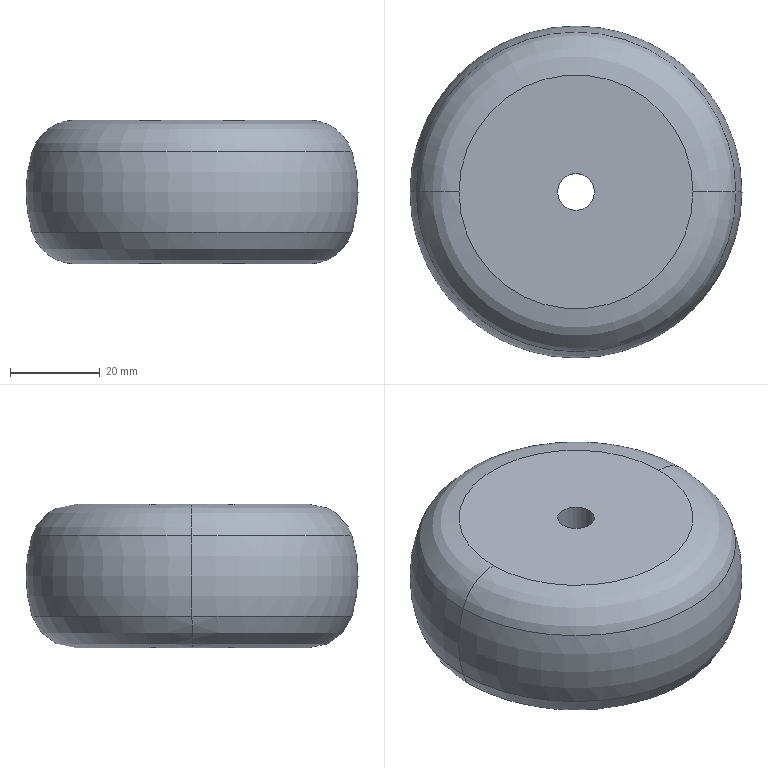Part | SolidWorks | features Fillet 1, Revolution 1 | 1 solid | 10 faces | box 74 x 74 x 32 mm | volume 122167 mm3 | torus 6 | cylinder 2 | plane 2 | commonest cylinder face diameters 8.2 x2
STEP:
#1=CARTESIAN_POINT('',(-35.618,0.,9.));
#2=VERTEX_POINT('',#1);
#3=CARTESIAN_POINT('',(35.618,0.,9.));
#4=VERTEX_POINT('',#3);
#5=CARTESIAN_POINT('',(0.,0.,9.));
#6=DIRECTION('',(0.,0.,-1.));
#7=DIRECTION('',(-1.,0.,0.));
#8=AXIS2_PLACEMENT_3D('',#5,#6,#7);
#9=CIRCLE('',#8,35.618);
#10=EDGE_CURVE('',#2,#4,#9,.T.);
#11=ORIENTED_EDGE('',*,*,#10,.F.);
#12=CARTESIAN_POINT('',(-26.079,0.,16.));
#13=VERTEX_POINT('',#12);
#14=CARTESIAN_POINT('',(-26.079,0.,6.));
#15=DIRECTION('',(0.,1.,0.));
#16=DIRECTION('',(-1.,0.,0.));
#17=AXIS2_PLACEMENT_3D('',#14,#15,#16);
#18=CIRCLE('',#17,10.);
#19=EDGE_CURVE('',#2,#13,#18,.T.);
#20=ORIENTED_EDGE('',*,*,#19,.T.);
#21=CARTESIAN_POINT('',(26.079,0.,16.));
#22=VERTEX_POINT('',#21);
#23=CARTESIAN_POINT('',(0.,0.,16.));
#24=DIRECTION('',(0.,0.,1.));
#25=DIRECTION('',(1.,0.,0.));
#26=AXIS2_PLACEMENT_3D('',#23,#24,#25);
#27=CIRCLE('',#26,26.079);
#28=EDGE_CURVE('',#22,#13,#27,.T.);
#29=ORIENTED_EDGE('',*,*,#28,.F.);
#30=CARTESIAN_POINT('',(26.079,0.,6.));
#31=DIRECTION('',(0.,-1.,0.));
#32=DIRECTION('',(0.,0.,-1.));
#33=AXIS2_PLACEMENT_3D('',#30,#31,#32);
#34=CIRCLE('',#33,10.);
#35=EDGE_CURVE('',#4,#22,#34,.T.);
#36=ORIENTED_EDGE('',*,*,#35,.F.);
#37=EDGE_LOOP('',(#11,#20,#29,#36));
#38=FACE_OUTER_BOUND('',#37,.T.);
#39=CARTESIAN_POINT('',(0.,0.,6.));
#40=DIRECTION('',(0.,0.,1.));
#41=DIRECTION('',(1.,0.,0.));
#42=AXIS2_PLACEMENT_3D('',#39,#40,#41);
#43=TOROIDAL_SURFACE('',#42,26.079,10.);
#44=ADVANCED_FACE('',(#38),#43,.T.);
#45=CARTESIAN_POINT('',(35.618,0.,-9.));
#46=VERTEX_POINT('',#45);
#47=CARTESIAN_POINT('',(-35.618,0.,-9.));
#48=VERTEX_POINT('',#47);
#49=CARTESIAN_POINT('',(0.,0.,-9.));
#50=DIRECTION('',(0.,0.,1.));
#51=DIRECTION('',(1.,0.,0.));
#52=AXIS2_PLACEMENT_3D('',#49,#50,#51);
#53=CIRCLE('',#52,35.618);
#54=EDGE_CURVE('',#46,#48,#53,.T.);
#55=ORIENTED_EDGE('',*,*,#54,.F.);
#56=CARTESIAN_POINT('',(26.079,0.,-16.));
#57=VERTEX_POINT('',#56);
#58=CARTESIAN_POINT('',(26.079,0.,-6.));
#59=DIRECTION('',(0.,1.,0.));
#60=DIRECTION('',(-1.,0.,0.));
#61=AXIS2_PLACEMENT_3D('',#58,#59,#60);
#62=CIRCLE('',#61,10.);
#63=EDGE_CURVE('',#46,#57,#62,.T.);
#64=ORIENTED_EDGE('',*,*,#63,.T.);
#65=CARTESIAN_POINT('',(-26.079,0.,-16.));
#66=VERTEX_POINT('',#65);
#67=CARTESIAN_POINT('',(0.,0.,-16.));
#68=DIRECTION('',(0.,0.,-1.));
#69=DIRECTION('',(-1.,0.,0.));
#70=AXIS2_PLACEMENT_3D('',#67,#68,#69);
#71=CIRCLE('',#70,26.079);
#72=EDGE_CURVE('',#66,#57,#71,.T.);
#73=ORIENTED_EDGE('',*,*,#72,.F.);
#74=CARTESIAN_POINT('',(-26.079,0.,-6.));
#75=DIRECTION('',(0.,-1.,0.));
#76=DIRECTION('',(0.,0.,-1.));
#77=AXIS2_PLACEMENT_3D('',#74,#75,#76);
#78=CIRCLE('',#77,10.);
#79=EDGE_CURVE('',#48,#66,#78,.T.);
#80=ORIENTED_EDGE('',*,*,#79,.F.);
#81=EDGE_LOOP('',(#55,#64,#73,#80));
#82=FACE_OUTER_BOUND('',#81,.T.);
#83=CARTESIAN_POINT('',(0.,0.,-6.));
#84=DIRECTION('',(0.,0.,-1.));
#85=DIRECTION('',(-1.,0.,0.));
#86=AXIS2_PLACEMENT_3D('',#83,#84,#85);
#87=TOROIDAL_SURFACE('',#86,26.079,10.);
#88=ADVANCED_FACE('',(#82),#87,.T.);
#89=ORIENTED_EDGE('',*,*,#54,.T.);
#90=CARTESIAN_POINT('',(-7.,0.,0.));
#91=DIRECTION('',(0.,1.,0.));
#92=DIRECTION('',(-1.,0.,0.));
#93=AXIS2_PLACEMENT_3D('',#90,#91,#92);
#94=CIRCLE('',#93,30.);
#95=EDGE_CURVE('',#48,#2,#94,.T.);
#96=ORIENTED_EDGE('',*,*,#95,.T.);
#97=ORIENTED_EDGE('',*,*,#10,.T.);
#98=CARTESIAN_POINT('',(7.,0.,0.));
#99=DIRECTION('',(0.,-1.,0.));
#100=DIRECTION('',(0.,0.,-1.));
#101=AXIS2_PLACEMENT_3D('',#98,#99,#100);
#102=CIRCLE('',#101,30.);
#103=EDGE_CURVE('',#46,#4,#102,.T.);
#104=ORIENTED_EDGE('',*,*,#103,.F.);
#105=EDGE_LOOP('',(#89,#96,#97,#104));
#106=FACE_OUTER_BOUND('',#105,.T.);
#107=CARTESIAN_POINT('',(0.,0.,0.));
#108=DIRECTION('',(0.,0.,1.));
#109=DIRECTION('',(1.,0.,0.));
#110=AXIS2_PLACEMENT_3D('',#107,#108,#109);
#111=TOROIDAL_SURFACE('',#110,7.,30.);
#112=ADVANCED_FACE('',(#106),#111,.T.);
#113=CARTESIAN_POINT('',(-4.1,0.,-16.));
#114=VERTEX_POINT('',#113);
#115=CARTESIAN_POINT('',(4.1,0.,-16.));
#116=VERTEX_POINT('',#115);
#117=CARTESIAN_POINT('',(0.,0.,-16.));
#118=DIRECTION('',(0.,0.,1.));
#119=DIRECTION('',(1.,0.,0.));
#120=AXIS2_PLACEMENT_3D('',#117,#118,#119);
#121=CIRCLE('',#120,4.1);
#122=EDGE_CURVE('',#114,#116,#121,.T.);
#123=ORIENTED_EDGE('',*,*,#122,.F.);
#124=CARTESIAN_POINT('',(-4.1,0.,16.));
#125=VERTEX_POINT('',#124);
#126=CARTESIAN_POINT('',(-4.1,0.,0.));
#127=DIRECTION('',(0.,0.,1.));
#128=VECTOR('',#127,1000.);
#129=LINE('',#126,#128);
#130=EDGE_CURVE('',#114,#125,#129,.T.);
#131=ORIENTED_EDGE('',*,*,#130,.T.);
#132=CARTESIAN_POINT('',(4.1,0.,16.));
#133=VERTEX_POINT('',#132);
#134=CARTESIAN_POINT('',(0.,0.,16.));
#135=DIRECTION('',(0.,0.,1.));
#136=DIRECTION('',(1.,0.,0.));
#137=AXIS2_PLACEMENT_3D('',#134,#135,#136);
#138=CIRCLE('',#137,4.1);
#139=EDGE_CURVE('',#125,#133,#138,.T.);
#140=ORIENTED_EDGE('',*,*,#139,.T.);
#141=CARTESIAN_POINT('',(4.1,0.,0.));
#142=DIRECTION('',(0.,0.,1.));
#143=VECTOR('',#142,1000.);
#144=LINE('',#141,#143);
#145=EDGE_CURVE('',#116,#133,#144,.T.);
#146=ORIENTED_EDGE('',*,*,#145,.F.);
#147=EDGE_LOOP('',(#123,#131,#140,#146));
#148=FACE_OUTER_BOUND('',#147,.T.);
#149=CARTESIAN_POINT('',(0.,0.,0.));
#150=DIRECTION('',(0.,0.,1.));
#151=DIRECTION('',(1.,0.,0.));
#152=AXIS2_PLACEMENT_3D('',#149,#150,#151);
#153=CYLINDRICAL_SURFACE('',#152,4.1);
#154=ADVANCED_FACE('',(#148),#153,.F.);
#155=ORIENTED_EDGE('',*,*,#130,.F.);
#156=CARTESIAN_POINT('',(0.,0.,-16.));
#157=DIRECTION('',(0.,0.,1.));
#158=DIRECTION('',(1.,0.,0.));
#159=AXIS2_PLACEMENT_3D('',#156,#157,#158);
#160=CIRCLE('',#159,4.1);
#161=EDGE_CURVE('',#116,#114,#160,.T.);
#162=ORIENTED_EDGE('',*,*,#161,.F.);
#163=ORIENTED_EDGE('',*,*,#145,.T.);
#164=CARTESIAN_POINT('',(0.,0.,16.));
#165=DIRECTION('',(0.,0.,1.));
#166=DIRECTION('',(1.,0.,0.));
#167=AXIS2_PLACEMENT_3D('',#164,#165,#166);
#168=CIRCLE('',#167,4.1);
#169=EDGE_CURVE('',#133,#125,#168,.T.);
#170=ORIENTED_EDGE('',*,*,#169,.T.);
#171=EDGE_LOOP('',(#155,#162,#163,#170));
#172=FACE_OUTER_BOUND('',#171,.T.);
#173=CARTESIAN_POINT('',(0.,0.,0.));
#174=DIRECTION('',(0.,0.,1.));
#175=DIRECTION('',(1.,0.,0.));
#176=AXIS2_PLACEMENT_3D('',#173,#174,#175);
#177=CYLINDRICAL_SURFACE('',#176,4.1);
#178=ADVANCED_FACE('',(#172),#177,.F.);
#179=ORIENTED_EDGE('',*,*,#72,.T.);
#180=CARTESIAN_POINT('',(0.,0.,-16.));
#181=DIRECTION('',(0.,0.,-1.));
#182=DIRECTION('',(-1.,0.,0.));
#183=AXIS2_PLACEMENT_3D('',#180,#181,#182);
#184=CIRCLE('',#183,26.079);
#185=EDGE_CURVE('',#57,#66,#184,.T.);
#186=ORIENTED_EDGE('',*,*,#185,.T.);
#187=EDGE_LOOP('',(#179,#186));
#188=FACE_OUTER_BOUND('',#187,.T.);
#189=ORIENTED_EDGE('',*,*,#161,.T.);
#190=ORIENTED_EDGE('',*,*,#122,.T.);
#191=EDGE_LOOP('',(#189,#190));
#192=FACE_BOUND('',#191,.T.);
#193=CARTESIAN_POINT('',(4.1,0.,-16.));
#194=DIRECTION('',(0.,0.,-1.));
#195=DIRECTION('',(-1.,0.,0.));
#196=AXIS2_PLACEMENT_3D('',#193,#194,#195);
#197=PLANE('',#196);
#198=ADVANCED_FACE('',(#188,#192),#197,.T.);
#199=ORIENTED_EDGE('',*,*,#95,.F.);
#200=CARTESIAN_POINT('',(0.,0.,-9.));
#201=DIRECTION('',(0.,0.,1.));
#202=DIRECTION('',(1.,0.,0.));
#203=AXIS2_PLACEMENT_3D('',#200,#201,#202);
#204=CIRCLE('',#203,35.618);
#205=EDGE_CURVE('',#48,#46,#204,.T.);
#206=ORIENTED_EDGE('',*,*,#205,.T.);
#207=ORIENTED_EDGE('',*,*,#103,.T.);
#208=CARTESIAN_POINT('',(0.,0.,9.));
#209=DIRECTION('',(0.,0.,-1.));
#210=DIRECTION('',(-1.,0.,0.));
#211=AXIS2_PLACEMENT_3D('',#208,#209,#210);
#212=CIRCLE('',#211,35.618);
#213=EDGE_CURVE('',#4,#2,#212,.T.);
#214=ORIENTED_EDGE('',*,*,#213,.T.);
#215=EDGE_LOOP('',(#199,#206,#207,#214));
#216=FACE_OUTER_BOUND('',#215,.T.);
#217=CARTESIAN_POINT('',(0.,0.,0.));
#218=DIRECTION('',(0.,0.,1.));
#219=DIRECTION('',(1.,0.,0.));
#220=AXIS2_PLACEMENT_3D('',#217,#218,#219);
#221=TOROIDAL_SURFACE('',#220,7.,30.);
#222=ADVANCED_FACE('',(#216),#221,.T.);
#223=ORIENTED_EDGE('',*,*,#28,.T.);
#224=CARTESIAN_POINT('',(0.,0.,16.));
#225=DIRECTION('',(0.,0.,1.));
#226=DIRECTION('',(1.,0.,0.));
#227=AXIS2_PLACEMENT_3D('',#224,#225,#226);
#228=CIRCLE('',#227,26.079);
#229=EDGE_CURVE('',#13,#22,#228,.T.);
#230=ORIENTED_EDGE('',*,*,#229,.T.);
#231=EDGE_LOOP('',(#223,#230));
#232=FACE_OUTER_BOUND('',#231,.T.);
#233=ORIENTED_EDGE('',*,*,#169,.F.);
#234=ORIENTED_EDGE('',*,*,#139,.F.);
#235=EDGE_LOOP('',(#233,#234));
#236=FACE_BOUND('',#235,.T.);
#237=CARTESIAN_POINT('',(4.1,0.,16.));
#238=DIRECTION('',(0.,0.,1.));
#239=DIRECTION('',(1.,0.,0.));
#240=AXIS2_PLACEMENT_3D('',#237,#238,#239);
#241=PLANE('',#240);
#242=ADVANCED_FACE('',(#232,#236),#241,.T.);
#243=ORIENTED_EDGE('',*,*,#63,.F.);
#244=ORIENTED_EDGE('',*,*,#205,.F.);
#245=ORIENTED_EDGE('',*,*,#79,.T.);
#246=ORIENTED_EDGE('',*,*,#185,.F.);
#247=EDGE_LOOP('',(#243,#244,#245,#246));
#248=FACE_OUTER_BOUND('',#247,.T.);
#249=CARTESIAN_POINT('',(0.,0.,-6.));
#250=DIRECTION('',(0.,0.,-1.));
#251=DIRECTION('',(-1.,0.,0.));
#252=AXIS2_PLACEMENT_3D('',#249,#250,#251);
#253=TOROIDAL_SURFACE('',#252,26.079,10.);
#254=ADVANCED_FACE('',(#248),#253,.T.);
#255=ORIENTED_EDGE('',*,*,#19,.F.);
#256=ORIENTED_EDGE('',*,*,#213,.F.);
#257=ORIENTED_EDGE('',*,*,#35,.T.);
#258=ORIENTED_EDGE('',*,*,#229,.F.);
#259=EDGE_LOOP('',(#255,#256,#257,#258));
#260=FACE_OUTER_BOUND('',#259,.T.);
#261=CARTESIAN_POINT('',(0.,0.,6.));
#262=DIRECTION('',(0.,0.,1.));
#263=DIRECTION('',(1.,0.,0.));
#264=AXIS2_PLACEMENT_3D('',#261,#262,#263);
#265=TOROIDAL_SURFACE('',#264,26.079,10.);
#266=ADVANCED_FACE('',(#260),#265,.T.);
#267=CLOSED_SHELL('',(#44,#88,#112,#154,#178,#198,#222,#242,#254,#266));
#268=MANIFOLD_SOLID_BREP('',#267);
#269=CARTESIAN_POINT('',(0.,0.,0.));
#270=DIRECTION('',(0.,0.,1.));
#271=DIRECTION('',(1.,0.,0.));
#272=AXIS2_PLACEMENT_3D('',#269,#270,#271);
#273=(LENGTH_UNIT()NAMED_UNIT(*)SI_UNIT(.MILLI.,.METRE.));
#274=UNCERTAINTY_MEASURE_WITH_UNIT(LENGTH_MEASURE(0.00001),#273,'','');
#275=(NAMED_UNIT(*)PLANE_ANGLE_UNIT()SI_UNIT($,.RADIAN.));
#276=(NAMED_UNIT(*)SI_UNIT($,.STERADIAN.)SOLID_ANGLE_UNIT());
#277=(GEOMETRIC_REPRESENTATION_CONTEXT(3)GLOBAL_UNCERTAINTY_ASSIGNED_CONTEXT((#274))GLOBAL_UNIT_ASSIGNED_CONTEXT((#273,#275,#276))REPRESENTATION_CONTEXT('',''));
#278=ADVANCED_BREP_SHAPE_REPRESENTATION('',(#268,#272),#277);